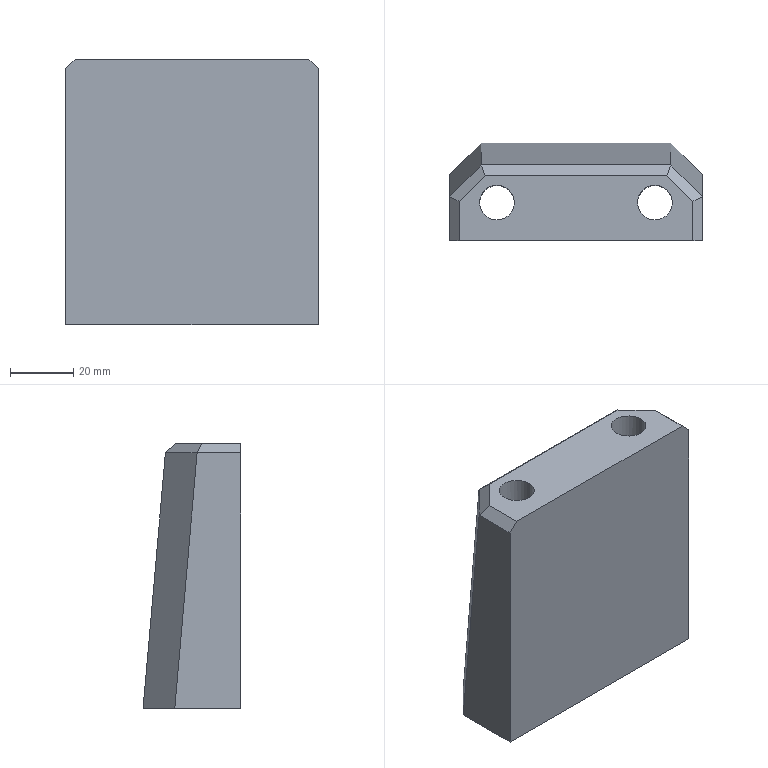Part | STEP file | P011002NF02-000 | 1 solid | 29 faces | box 80 x 31 x 84 mm | volume 154459 mm3 | plane 13 | cylinder 7 | spline 6 | cone 3 | commonest cylinder face diameters 11 x2 17 x2 8.5 x1 9.967 x1 10 x1